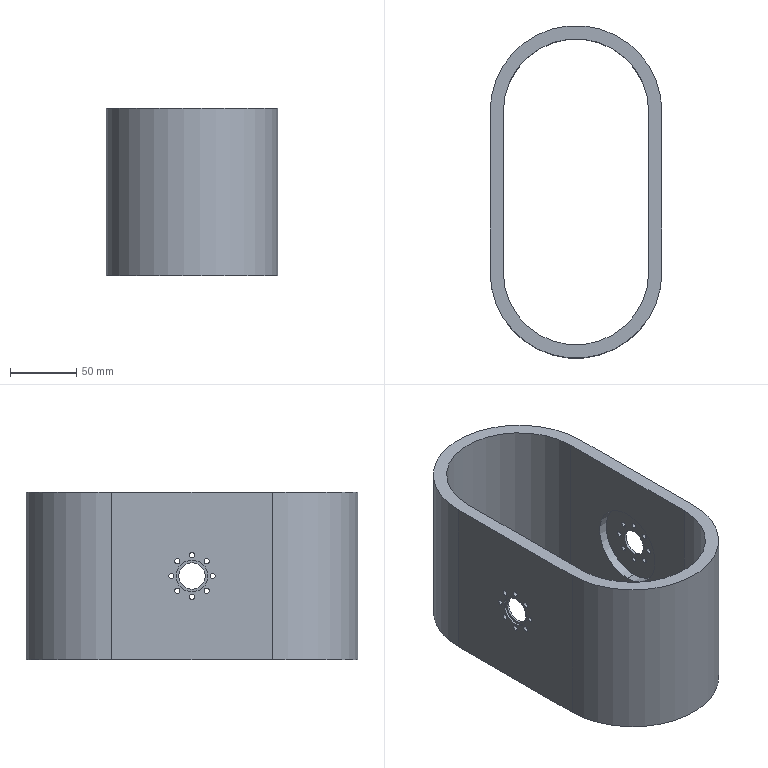Part | SolidWorks | features ICE 4, SavedExtBody 1 | 1 solid | 58 faces | box 130 x 251.564 x 126.792 mm | volume 744560 mm3 | cylinder 48 | plane 10 | commonest cylinder face diameters 4 x32 20 x4 24 x4 59.401 x4 110 x2 130 x2